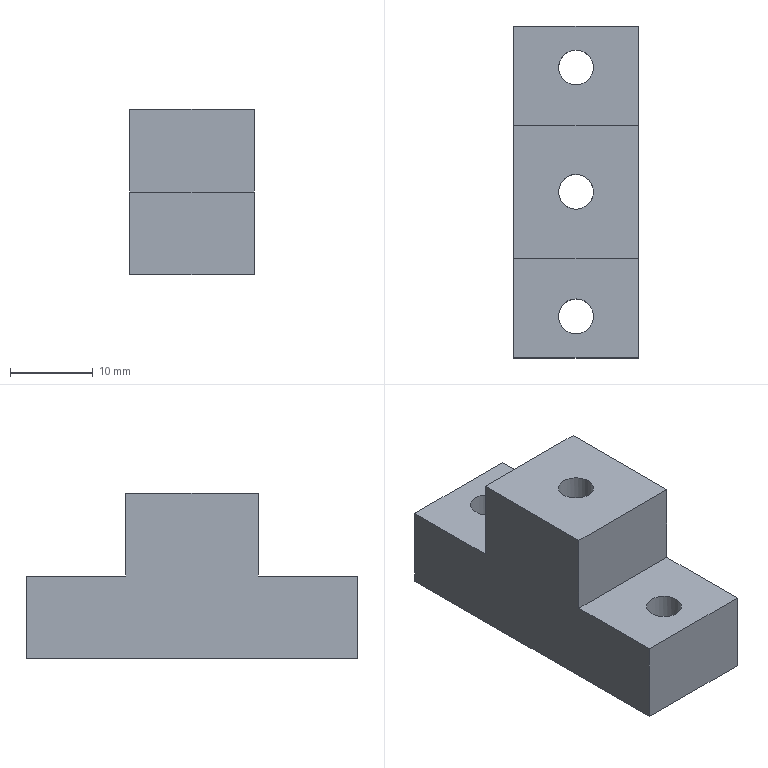Part | NX | features DATUM_CSYS 4, SKETCH 3, EXTRUDE 2, CBORE_HOLE 1, HOLE PACKAGE 1 | 1 solid | 15 faces | box 15 x 40 x 20 mm | volume 7409 mm3 | plane 11 | cylinder 4 | commonest cylinder face diameters 4.2 x3 8 x1
STEP:
#1=CARTESIAN_POINT('',(0.,-20.,10.));
#2=VERTEX_POINT('',#1);
#3=CARTESIAN_POINT('',(0.,-20.,0.));
#4=VERTEX_POINT('',#3);
#5=CARTESIAN_POINT('',(0.,-20.,10.));
#6=DIRECTION('',(0.,0.,-1.));
#7=VECTOR('',#6,1000.);
#8=LINE('',#5,#7);
#9=EDGE_CURVE('',#2,#4,#8,.T.);
#10=ORIENTED_EDGE('',*,*,#9,.T.);
#11=CARTESIAN_POINT('',(15.,-20.,0.));
#12=VERTEX_POINT('',#11);
#13=CARTESIAN_POINT('',(15.,-20.,0.));
#14=DIRECTION('',(-1.,0.,0.));
#15=VECTOR('',#14,1000.);
#16=LINE('',#13,#15);
#17=EDGE_CURVE('',#12,#4,#16,.T.);
#18=ORIENTED_EDGE('',*,*,#17,.F.);
#19=CARTESIAN_POINT('',(15.,-20.,10.));
#20=VERTEX_POINT('',#19);
#21=CARTESIAN_POINT('',(15.,-20.,10.));
#22=DIRECTION('',(0.,0.,-1.));
#23=VECTOR('',#22,1000.);
#24=LINE('',#21,#23);
#25=EDGE_CURVE('',#20,#12,#24,.T.);
#26=ORIENTED_EDGE('',*,*,#25,.F.);
#27=CARTESIAN_POINT('',(15.,-20.,10.));
#28=DIRECTION('',(-1.,0.,0.));
#29=VECTOR('',#28,1000.);
#30=LINE('',#27,#29);
#31=EDGE_CURVE('',#20,#2,#30,.T.);
#32=ORIENTED_EDGE('',*,*,#31,.T.);
#33=EDGE_LOOP('',(#10,#18,#26,#32));
#34=FACE_BOUND('',#33,.T.);
#35=CARTESIAN_POINT('',(15.,-20.,10.));
#36=DIRECTION('',(0.,1.,0.));
#37=DIRECTION('',(0.,0.,1.));
#38=AXIS2_PLACEMENT_3D('',#35,#36,#37);
#39=PLANE('',#38);
#40=ADVANCED_FACE('',(#34),#39,.F.);
#41=CARTESIAN_POINT('',(11.5,0.,0.));
#42=VERTEX_POINT('',#41);
#43=CARTESIAN_POINT('',(7.5,0.,0.));
#44=DIRECTION('',(0.,0.,1.));
#45=DIRECTION('',(1.,0.,0.));
#46=AXIS2_PLACEMENT_3D('',#43,#44,#45);
#47=CIRCLE('',#46,4.);
#48=EDGE_CURVE('',#42,#42,#47,.T.);
#49=ORIENTED_EDGE('',*,*,#48,.T.);
#50=EDGE_LOOP('',(#49));
#51=FACE_BOUND('',#50,.T.);
#52=CARTESIAN_POINT('',(9.6,15.,0.));
#53=VERTEX_POINT('',#52);
#54=CARTESIAN_POINT('',(7.5,15.,0.));
#55=DIRECTION('',(0.,0.,1.));
#56=DIRECTION('',(1.,0.,0.));
#57=AXIS2_PLACEMENT_3D('',#54,#55,#56);
#58=CIRCLE('',#57,2.1);
#59=EDGE_CURVE('',#53,#53,#58,.T.);
#60=ORIENTED_EDGE('',*,*,#59,.T.);
#61=EDGE_LOOP('',(#60));
#62=FACE_BOUND('',#61,.T.);
#63=CARTESIAN_POINT('',(9.6,-15.,0.));
#64=VERTEX_POINT('',#63);
#65=CARTESIAN_POINT('',(7.5,-15.,0.));
#66=DIRECTION('',(0.,0.,1.));
#67=DIRECTION('',(1.,0.,0.));
#68=AXIS2_PLACEMENT_3D('',#65,#66,#67);
#69=CIRCLE('',#68,2.1);
#70=EDGE_CURVE('',#64,#64,#69,.T.);
#71=ORIENTED_EDGE('',*,*,#70,.T.);
#72=EDGE_LOOP('',(#71));
#73=FACE_BOUND('',#72,.T.);
#74=CARTESIAN_POINT('',(0.,20.,0.));
#75=VERTEX_POINT('',#74);
#76=CARTESIAN_POINT('',(0.,0.,0.));
#77=DIRECTION('',(0.,1.,0.));
#78=VECTOR('',#77,1000.);
#79=LINE('',#76,#78);
#80=EDGE_CURVE('',#4,#75,#79,.T.);
#81=ORIENTED_EDGE('',*,*,#80,.T.);
#82=CARTESIAN_POINT('',(15.,20.,0.));
#83=VERTEX_POINT('',#82);
#84=CARTESIAN_POINT('',(15.,20.,0.));
#85=DIRECTION('',(-1.,0.,0.));
#86=VECTOR('',#85,1000.);
#87=LINE('',#84,#86);
#88=EDGE_CURVE('',#83,#75,#87,.T.);
#89=ORIENTED_EDGE('',*,*,#88,.F.);
#90=CARTESIAN_POINT('',(15.,-20.,0.));
#91=DIRECTION('',(0.,1.,0.));
#92=VECTOR('',#91,1000.);
#93=LINE('',#90,#92);
#94=EDGE_CURVE('',#12,#83,#93,.T.);
#95=ORIENTED_EDGE('',*,*,#94,.F.);
#96=ORIENTED_EDGE('',*,*,#17,.T.);
#97=EDGE_LOOP('',(#81,#89,#95,#96));
#98=FACE_BOUND('',#97,.T.);
#99=CARTESIAN_POINT('',(15.,0.,0.));
#100=DIRECTION('',(0.,0.,1.));
#101=DIRECTION('',(1.,0.,0.));
#102=AXIS2_PLACEMENT_3D('',#99,#100,#101);
#103=PLANE('',#102);
#104=ADVANCED_FACE('',(#51,#62,#73,#98),#103,.F.);
#105=CARTESIAN_POINT('',(0.,20.,10.));
#106=VERTEX_POINT('',#105);
#107=CARTESIAN_POINT('',(0.,20.,0.));
#108=DIRECTION('',(0.,0.,1.));
#109=VECTOR('',#108,1000.);
#110=LINE('',#107,#109);
#111=EDGE_CURVE('',#75,#106,#110,.T.);
#112=ORIENTED_EDGE('',*,*,#111,.T.);
#113=CARTESIAN_POINT('',(15.,20.,10.));
#114=VERTEX_POINT('',#113);
#115=CARTESIAN_POINT('',(15.,20.,10.));
#116=DIRECTION('',(-1.,0.,0.));
#117=VECTOR('',#116,1000.);
#118=LINE('',#115,#117);
#119=EDGE_CURVE('',#114,#106,#118,.T.);
#120=ORIENTED_EDGE('',*,*,#119,.F.);
#121=CARTESIAN_POINT('',(15.,20.,0.));
#122=DIRECTION('',(0.,0.,1.));
#123=VECTOR('',#122,1000.);
#124=LINE('',#121,#123);
#125=EDGE_CURVE('',#83,#114,#124,.T.);
#126=ORIENTED_EDGE('',*,*,#125,.F.);
#127=ORIENTED_EDGE('',*,*,#88,.T.);
#128=EDGE_LOOP('',(#112,#120,#126,#127));
#129=FACE_BOUND('',#128,.T.);
#130=CARTESIAN_POINT('',(15.,20.,0.));
#131=DIRECTION('',(0.,-1.,0.));
#132=DIRECTION('',(0.,0.,-1.));
#133=AXIS2_PLACEMENT_3D('',#130,#131,#132);
#134=PLANE('',#133);
#135=ADVANCED_FACE('',(#129),#134,.F.);
#136=CARTESIAN_POINT('',(7.5,17.1,10.));
#137=VERTEX_POINT('',#136);
#138=CARTESIAN_POINT('',(7.5,15.,10.));
#139=DIRECTION('',(0.,0.,-1.));
#140=DIRECTION('',(0.,1.,0.));
#141=AXIS2_PLACEMENT_3D('',#138,#139,#140);
#142=CIRCLE('',#141,2.1);
#143=EDGE_CURVE('',#137,#137,#142,.F.);
#144=ORIENTED_EDGE('',*,*,#143,.F.);
#145=EDGE_LOOP('',(#144));
#146=FACE_BOUND('',#145,.T.);
#147=CARTESIAN_POINT('',(0.,8.,10.));
#148=VERTEX_POINT('',#147);
#149=CARTESIAN_POINT('',(0.,20.,10.));
#150=DIRECTION('',(0.,-1.,0.));
#151=VECTOR('',#150,1000.);
#152=LINE('',#149,#151);
#153=EDGE_CURVE('',#106,#148,#152,.T.);
#154=ORIENTED_EDGE('',*,*,#153,.T.);
#155=CARTESIAN_POINT('',(15.,8.,10.));
#156=VERTEX_POINT('',#155);
#157=CARTESIAN_POINT('',(15.,8.,10.));
#158=DIRECTION('',(-1.,0.,0.));
#159=VECTOR('',#158,1000.);
#160=LINE('',#157,#159);
#161=EDGE_CURVE('',#156,#148,#160,.T.);
#162=ORIENTED_EDGE('',*,*,#161,.F.);
#163=CARTESIAN_POINT('',(15.,20.,10.));
#164=DIRECTION('',(0.,-1.,0.));
#165=VECTOR('',#164,1000.);
#166=LINE('',#163,#165);
#167=EDGE_CURVE('',#114,#156,#166,.T.);
#168=ORIENTED_EDGE('',*,*,#167,.F.);
#169=ORIENTED_EDGE('',*,*,#119,.T.);
#170=EDGE_LOOP('',(#154,#162,#168,#169));
#171=FACE_BOUND('',#170,.T.);
#172=CARTESIAN_POINT('',(15.,20.,10.));
#173=DIRECTION('',(0.,0.,-1.));
#174=DIRECTION('',(0.,1.,0.));
#175=AXIS2_PLACEMENT_3D('',#172,#173,#174);
#176=PLANE('',#175);
#177=ADVANCED_FACE('',(#146,#171),#176,.F.);
#178=CARTESIAN_POINT('',(0.,8.,20.));
#179=VERTEX_POINT('',#178);
#180=CARTESIAN_POINT('',(0.,8.,10.));
#181=DIRECTION('',(0.,0.,1.));
#182=VECTOR('',#181,1000.);
#183=LINE('',#180,#182);
#184=EDGE_CURVE('',#148,#179,#183,.T.);
#185=ORIENTED_EDGE('',*,*,#184,.T.);
#186=CARTESIAN_POINT('',(15.,8.,20.));
#187=VERTEX_POINT('',#186);
#188=CARTESIAN_POINT('',(15.,8.,20.));
#189=DIRECTION('',(-1.,0.,0.));
#190=VECTOR('',#189,1000.);
#191=LINE('',#188,#190);
#192=EDGE_CURVE('',#187,#179,#191,.T.);
#193=ORIENTED_EDGE('',*,*,#192,.F.);
#194=CARTESIAN_POINT('',(15.,8.,10.));
#195=DIRECTION('',(0.,0.,1.));
#196=VECTOR('',#195,1000.);
#197=LINE('',#194,#196);
#198=EDGE_CURVE('',#156,#187,#197,.T.);
#199=ORIENTED_EDGE('',*,*,#198,.F.);
#200=ORIENTED_EDGE('',*,*,#161,.T.);
#201=EDGE_LOOP('',(#185,#193,#199,#200));
#202=FACE_BOUND('',#201,.T.);
#203=CARTESIAN_POINT('',(15.,8.,10.));
#204=DIRECTION('',(0.,-1.,0.));
#205=DIRECTION('',(0.,0.,-1.));
#206=AXIS2_PLACEMENT_3D('',#203,#204,#205);
#207=PLANE('',#206);
#208=ADVANCED_FACE('',(#202),#207,.F.);
#209=CARTESIAN_POINT('',(7.5,2.1,20.));
#210=VERTEX_POINT('',#209);
#211=CARTESIAN_POINT('',(7.5,0.,20.));
#212=DIRECTION('',(0.,0.,-1.));
#213=DIRECTION('',(0.,1.,0.));
#214=AXIS2_PLACEMENT_3D('',#211,#212,#213);
#215=CIRCLE('',#214,2.1);
#216=EDGE_CURVE('',#210,#210,#215,.T.);
#217=ORIENTED_EDGE('',*,*,#216,.T.);
#218=EDGE_LOOP('',(#217));
#219=FACE_BOUND('',#218,.T.);
#220=CARTESIAN_POINT('',(0.,-8.,20.));
#221=VERTEX_POINT('',#220);
#222=CARTESIAN_POINT('',(0.,0.,20.));
#223=DIRECTION('',(0.,-1.,0.));
#224=VECTOR('',#223,1000.);
#225=LINE('',#222,#224);
#226=EDGE_CURVE('',#179,#221,#225,.T.);
#227=ORIENTED_EDGE('',*,*,#226,.T.);
#228=CARTESIAN_POINT('',(15.,-8.,20.));
#229=VERTEX_POINT('',#228);
#230=CARTESIAN_POINT('',(15.,-8.,20.));
#231=DIRECTION('',(-1.,0.,0.));
#232=VECTOR('',#231,1000.);
#233=LINE('',#230,#232);
#234=EDGE_CURVE('',#229,#221,#233,.T.);
#235=ORIENTED_EDGE('',*,*,#234,.F.);
#236=CARTESIAN_POINT('',(15.,8.,20.));
#237=DIRECTION('',(0.,-1.,0.));
#238=VECTOR('',#237,1000.);
#239=LINE('',#236,#238);
#240=EDGE_CURVE('',#187,#229,#239,.T.);
#241=ORIENTED_EDGE('',*,*,#240,.F.);
#242=ORIENTED_EDGE('',*,*,#192,.T.);
#243=EDGE_LOOP('',(#227,#235,#241,#242));
#244=FACE_BOUND('',#243,.T.);
#245=CARTESIAN_POINT('',(15.,0.,20.));
#246=DIRECTION('',(0.,0.,-1.));
#247=DIRECTION('',(0.,1.,0.));
#248=AXIS2_PLACEMENT_3D('',#245,#246,#247);
#249=PLANE('',#248);
#250=ADVANCED_FACE('',(#219,#244),#249,.F.);
#251=CARTESIAN_POINT('',(0.,-8.,10.));
#252=VERTEX_POINT('',#251);
#253=CARTESIAN_POINT('',(0.,-8.,20.));
#254=DIRECTION('',(0.,0.,-1.));
#255=VECTOR('',#254,1000.);
#256=LINE('',#253,#255);
#257=EDGE_CURVE('',#221,#252,#256,.T.);
#258=ORIENTED_EDGE('',*,*,#257,.T.);
#259=CARTESIAN_POINT('',(15.,-8.,10.));
#260=VERTEX_POINT('',#259);
#261=CARTESIAN_POINT('',(15.,-8.,10.));
#262=DIRECTION('',(-1.,0.,0.));
#263=VECTOR('',#262,1000.);
#264=LINE('',#261,#263);
#265=EDGE_CURVE('',#260,#252,#264,.T.);
#266=ORIENTED_EDGE('',*,*,#265,.F.);
#267=CARTESIAN_POINT('',(15.,-8.,20.));
#268=DIRECTION('',(0.,0.,-1.));
#269=VECTOR('',#268,1000.);
#270=LINE('',#267,#269);
#271=EDGE_CURVE('',#229,#260,#270,.T.);
#272=ORIENTED_EDGE('',*,*,#271,.F.);
#273=ORIENTED_EDGE('',*,*,#234,.T.);
#274=EDGE_LOOP('',(#258,#266,#272,#273));
#275=FACE_BOUND('',#274,.T.);
#276=CARTESIAN_POINT('',(15.,-8.,20.));
#277=DIRECTION('',(0.,1.,0.));
#278=DIRECTION('',(0.,0.,1.));
#279=AXIS2_PLACEMENT_3D('',#276,#277,#278);
#280=PLANE('',#279);
#281=ADVANCED_FACE('',(#275),#280,.F.);
#282=CARTESIAN_POINT('',(7.5,-12.9,10.));
#283=VERTEX_POINT('',#282);
#284=CARTESIAN_POINT('',(7.5,-15.,10.));
#285=DIRECTION('',(0.,0.,-1.));
#286=DIRECTION('',(0.,1.,0.));
#287=AXIS2_PLACEMENT_3D('',#284,#285,#286);
#288=CIRCLE('',#287,2.1);
#289=EDGE_CURVE('',#283,#283,#288,.F.);
#290=ORIENTED_EDGE('',*,*,#289,.F.);
#291=EDGE_LOOP('',(#290));
#292=FACE_BOUND('',#291,.T.);
#293=CARTESIAN_POINT('',(0.,-8.,10.));
#294=DIRECTION('',(0.,-1.,0.));
#295=VECTOR('',#294,1000.);
#296=LINE('',#293,#295);
#297=EDGE_CURVE('',#252,#2,#296,.T.);
#298=ORIENTED_EDGE('',*,*,#297,.T.);
#299=ORIENTED_EDGE('',*,*,#31,.F.);
#300=CARTESIAN_POINT('',(15.,-8.,10.));
#301=DIRECTION('',(0.,-1.,0.));
#302=VECTOR('',#301,1000.);
#303=LINE('',#300,#302);
#304=EDGE_CURVE('',#260,#20,#303,.T.);
#305=ORIENTED_EDGE('',*,*,#304,.F.);
#306=ORIENTED_EDGE('',*,*,#265,.T.);
#307=EDGE_LOOP('',(#298,#299,#305,#306));
#308=FACE_BOUND('',#307,.T.);
#309=CARTESIAN_POINT('',(15.,-8.,10.));
#310=DIRECTION('',(0.,0.,-1.));
#311=DIRECTION('',(0.,1.,0.));
#312=AXIS2_PLACEMENT_3D('',#309,#310,#311);
#313=PLANE('',#312);
#314=ADVANCED_FACE('',(#292,#308),#313,.F.);
#315=ORIENTED_EDGE('',*,*,#25,.T.);
#316=ORIENTED_EDGE('',*,*,#94,.T.);
#317=ORIENTED_EDGE('',*,*,#125,.T.);
#318=ORIENTED_EDGE('',*,*,#167,.T.);
#319=ORIENTED_EDGE('',*,*,#198,.T.);
#320=ORIENTED_EDGE('',*,*,#240,.T.);
#321=ORIENTED_EDGE('',*,*,#271,.T.);
#322=ORIENTED_EDGE('',*,*,#304,.T.);
#323=EDGE_LOOP('',(#315,#316,#317,#318,#319,#320,#321,#322));
#324=FACE_BOUND('',#323,.T.);
#325=CARTESIAN_POINT('',(15.,0.,0.));
#326=DIRECTION('',(1.,0.,0.));
#327=DIRECTION('',(0.,0.,-1.));
#328=AXIS2_PLACEMENT_3D('',#325,#326,#327);
#329=PLANE('',#328);
#330=ADVANCED_FACE('',(#324),#329,.T.);
#331=ORIENTED_EDGE('',*,*,#9,.F.);
#332=ORIENTED_EDGE('',*,*,#297,.F.);
#333=ORIENTED_EDGE('',*,*,#257,.F.);
#334=ORIENTED_EDGE('',*,*,#226,.F.);
#335=ORIENTED_EDGE('',*,*,#184,.F.);
#336=ORIENTED_EDGE('',*,*,#153,.F.);
#337=ORIENTED_EDGE('',*,*,#111,.F.);
#338=ORIENTED_EDGE('',*,*,#80,.F.);
#339=EDGE_LOOP('',(#331,#332,#333,#334,#335,#336,#337,#338));
#340=FACE_BOUND('',#339,.T.);
#341=CARTESIAN_POINT('',(0.,0.,0.));
#342=DIRECTION('',(1.,0.,0.));
#343=DIRECTION('',(0.,0.,-1.));
#344=AXIS2_PLACEMENT_3D('',#341,#342,#343);
#345=PLANE('',#344);
#346=ADVANCED_FACE('',(#340),#345,.F.);
#347=ORIENTED_EDGE('',*,*,#70,.F.);
#348=EDGE_LOOP('',(#347));
#349=FACE_BOUND('',#348,.T.);
#350=ORIENTED_EDGE('',*,*,#289,.T.);
#351=EDGE_LOOP('',(#350));
#352=FACE_BOUND('',#351,.T.);
#353=CARTESIAN_POINT('',(7.5,-15.,15.));
#354=DIRECTION('',(0.,0.,-1.));
#355=DIRECTION('',(-1.,0.,0.));
#356=AXIS2_PLACEMENT_3D('',#353,#354,#355);
#357=CYLINDRICAL_SURFACE('',#356,2.1);
#358=ADVANCED_FACE('',(#349,#352),#357,.F.);
#359=ORIENTED_EDGE('',*,*,#59,.F.);
#360=EDGE_LOOP('',(#359));
#361=FACE_BOUND('',#360,.T.);
#362=ORIENTED_EDGE('',*,*,#143,.T.);
#363=EDGE_LOOP('',(#362));
#364=FACE_BOUND('',#363,.T.);
#365=CARTESIAN_POINT('',(7.5,15.,15.));
#366=DIRECTION('',(0.,0.,-1.));
#367=DIRECTION('',(-1.,0.,0.));
#368=AXIS2_PLACEMENT_3D('',#365,#366,#367);
#369=CYLINDRICAL_SURFACE('',#368,2.1);
#370=ADVANCED_FACE('',(#361,#364),#369,.F.);
#371=CARTESIAN_POINT('',(9.6,0.,12.));
#372=VERTEX_POINT('',#371);
#373=CARTESIAN_POINT('',(7.5,0.,12.));
#374=DIRECTION('',(0.,0.,1.));
#375=DIRECTION('',(1.,0.,0.));
#376=AXIS2_PLACEMENT_3D('',#373,#374,#375);
#377=CIRCLE('',#376,2.1);
#378=EDGE_CURVE('',#372,#372,#377,.F.);
#379=ORIENTED_EDGE('',*,*,#378,.T.);
#380=EDGE_LOOP('',(#379));
#381=FACE_BOUND('',#380,.T.);
#382=ORIENTED_EDGE('',*,*,#216,.F.);
#383=EDGE_LOOP('',(#382));
#384=FACE_BOUND('',#383,.T.);
#385=CARTESIAN_POINT('',(7.5,0.,50.));
#386=DIRECTION('',(0.,0.,1.));
#387=DIRECTION('',(1.,0.,0.));
#388=AXIS2_PLACEMENT_3D('',#385,#386,#387);
#389=CYLINDRICAL_SURFACE('',#388,2.1);
#390=ADVANCED_FACE('',(#381,#384),#389,.F.);
#391=ORIENTED_EDGE('',*,*,#378,.F.);
#392=EDGE_LOOP('',(#391));
#393=FACE_BOUND('',#392,.T.);
#394=CARTESIAN_POINT('',(11.5,0.,12.));
#395=VERTEX_POINT('',#394);
#396=CARTESIAN_POINT('',(7.5,0.,12.));
#397=DIRECTION('',(0.,0.,1.));
#398=DIRECTION('',(1.,0.,0.));
#399=AXIS2_PLACEMENT_3D('',#396,#397,#398);
#400=CIRCLE('',#399,4.);
#401=EDGE_CURVE('',#395,#395,#400,.F.);
#402=ORIENTED_EDGE('',*,*,#401,.T.);
#403=EDGE_LOOP('',(#402));
#404=FACE_BOUND('',#403,.T.);
#405=CARTESIAN_POINT('',(7.5,0.,12.));
#406=DIRECTION('',(0.,0.,1.));
#407=DIRECTION('',(1.,0.,0.));
#408=AXIS2_PLACEMENT_3D('',#405,#406,#407);
#409=PLANE('',#408);
#410=ADVANCED_FACE('',(#393,#404),#409,.F.);
#411=ORIENTED_EDGE('',*,*,#401,.F.);
#412=EDGE_LOOP('',(#411));
#413=FACE_BOUND('',#412,.T.);
#414=ORIENTED_EDGE('',*,*,#48,.F.);
#415=EDGE_LOOP('',(#414));
#416=FACE_BOUND('',#415,.T.);
#417=CARTESIAN_POINT('',(7.5,0.,0.));
#418=DIRECTION('',(0.,0.,1.));
#419=DIRECTION('',(1.,0.,0.));
#420=AXIS2_PLACEMENT_3D('',#417,#418,#419);
#421=CYLINDRICAL_SURFACE('',#420,4.);
#422=ADVANCED_FACE('',(#413,#416),#421,.F.);
#423=CLOSED_SHELL('',(#40,#104,#135,#177,#208,#250,#281,#314,#330,#346,#358,#370,#390,#410,#422));
#424=MANIFOLD_SOLID_BREP('',#423);
#425=(LENGTH_UNIT()NAMED_UNIT(*)SI_UNIT(.MILLI.,.METRE.));
#426=UNCERTAINTY_MEASURE_WITH_UNIT(LENGTH_MEASURE(0.00001),#425,'','');
#427=(NAMED_UNIT(*)PLANE_ANGLE_UNIT()SI_UNIT($,.RADIAN.));
#428=(NAMED_UNIT(*)SI_UNIT($,.STERADIAN.)SOLID_ANGLE_UNIT());
#429=(GEOMETRIC_REPRESENTATION_CONTEXT(3)GLOBAL_UNCERTAINTY_ASSIGNED_CONTEXT((#426))GLOBAL_UNIT_ASSIGNED_CONTEXT((#425,#427,#428))REPRESENTATION_CONTEXT('',''));
#430=ADVANCED_BREP_SHAPE_REPRESENTATION('',(#424),#429);